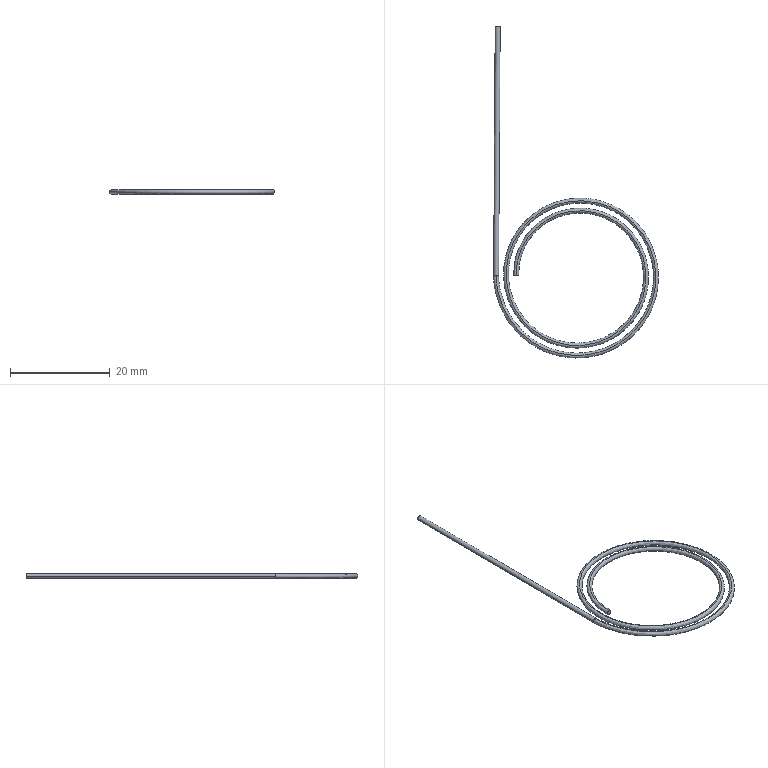Part | SolidWorks | features Helix 1, ICE 1, Sweep 1 | 1 solid | 6 faces | box 33.004 x 66.506 x 1 mm | volume 182.398 mm3 | cylinder 2 | spline 2 | plane 2 | commonest cylinder face diameters 1 x2